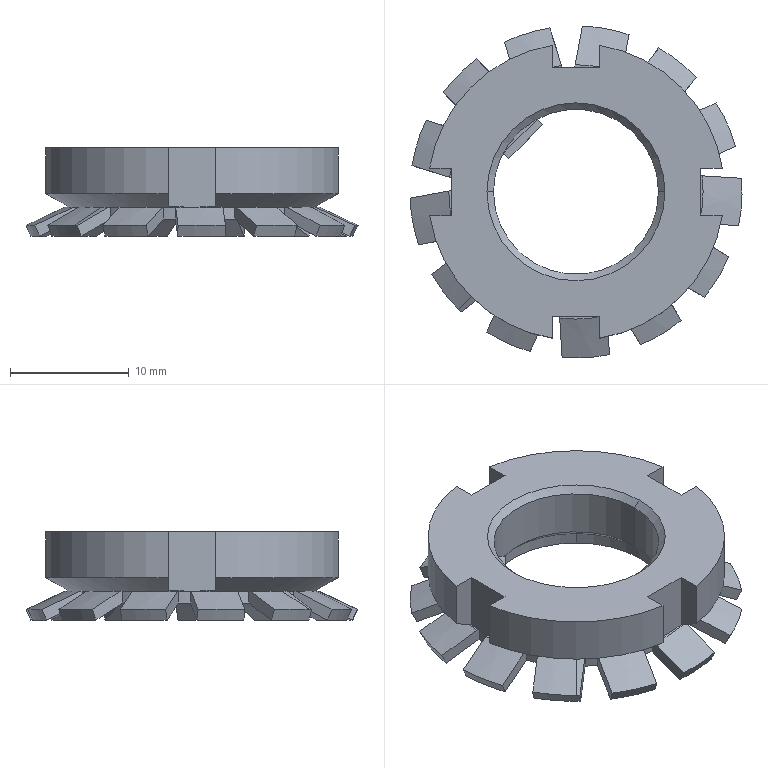Part | STEP file | Lock nut MISUMI JLNK15-1 | 2 solids | 119 faces | box 27.99 x 27.99 x 7.435 mm | volume 1826 mm3 | cone 50 | plane 47 | cylinder 22 | commonest cylinder face diameters 21 x13 25 x4 15 x3 13.917 x2